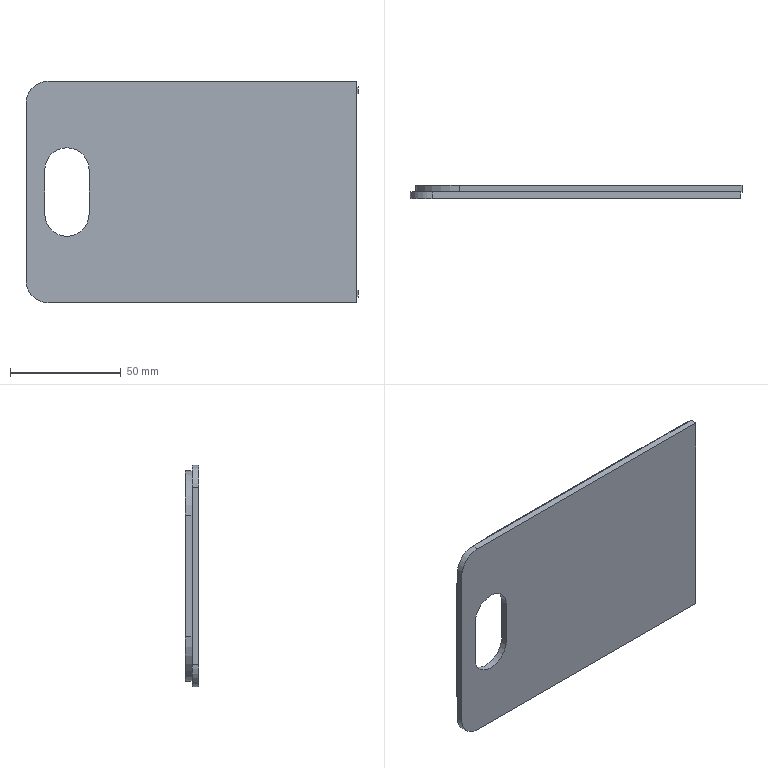Part | STEP file | 301 water tank cover | 1 solid | 29 faces | box 150 x 6 x 100 mm | volume 46035 mm3 | plane 20 | cylinder 9 | commonest cylinder face diameters 20 x5 40 x4